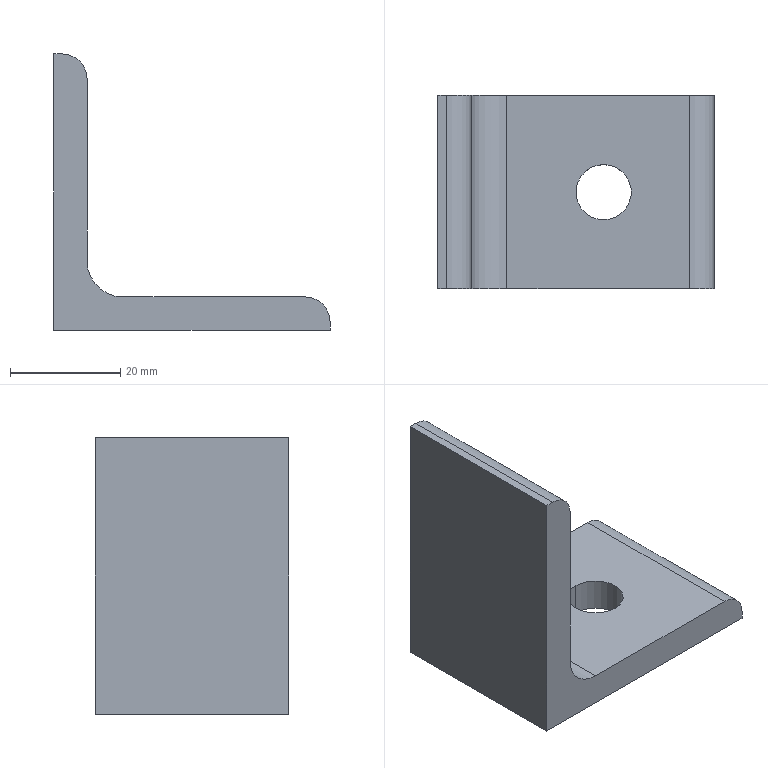Part | STEP file | [19]-2 | 1 solid | 13 faces | box 50 x 35 x 50 mm | volume 19282 mm3 | plane 8 | cylinder 5 | commonest cylinder face diameters 9 x2 10 x2 13 x1
STEP:
#1=CARTESIAN_POINT('',(30.,22.5,0.));
#2=VERTEX_POINT('',#1);
#3=CARTESIAN_POINT('',(30.,12.5,0.));
#4=VERTEX_POINT('',#3);
#5=CARTESIAN_POINT('',(30.,17.5,0.));
#6=DIRECTION('',(0.,0.,1.));
#7=DIRECTION('',(0.,-1.,0.));
#8=AXIS2_PLACEMENT_3D('',#5,#6,#7);
#9=CIRCLE('',#8,5.);
#10=EDGE_CURVE('',#2,#4,#9,.T.);
#11=ORIENTED_EDGE('',*,*,#10,.F.);
#12=CARTESIAN_POINT('',(30.,22.5,6.));
#13=VERTEX_POINT('',#12);
#14=CARTESIAN_POINT('',(30.,22.5,0.));
#15=DIRECTION('',(0.,0.,1.));
#16=VECTOR('',#15,1000.);
#17=LINE('',#14,#16);
#18=EDGE_CURVE('',#2,#13,#17,.T.);
#19=ORIENTED_EDGE('',*,*,#18,.T.);
#20=CARTESIAN_POINT('',(30.,12.5,6.));
#21=VERTEX_POINT('',#20);
#22=CARTESIAN_POINT('',(30.,17.5,6.));
#23=DIRECTION('',(0.,0.,-1.));
#24=DIRECTION('',(0.,1.,0.));
#25=AXIS2_PLACEMENT_3D('',#22,#23,#24);
#26=CIRCLE('',#25,5.);
#27=EDGE_CURVE('',#21,#13,#26,.T.);
#28=ORIENTED_EDGE('',*,*,#27,.F.);
#29=CARTESIAN_POINT('',(30.,12.5,0.));
#30=DIRECTION('',(0.,0.,1.));
#31=VECTOR('',#30,1000.);
#32=LINE('',#29,#31);
#33=EDGE_CURVE('',#4,#21,#32,.T.);
#34=ORIENTED_EDGE('',*,*,#33,.F.);
#35=EDGE_LOOP('',(#11,#19,#28,#34));
#36=FACE_OUTER_BOUND('',#35,.T.);
#37=CARTESIAN_POINT('',(30.,17.5,0.));
#38=DIRECTION('',(0.,0.,1.));
#39=DIRECTION('',(0.,-1.,0.));
#40=AXIS2_PLACEMENT_3D('',#37,#38,#39);
#41=CYLINDRICAL_SURFACE('',#40,5.);
#42=ADVANCED_FACE('',(#36),#41,.F.);
#43=CARTESIAN_POINT('',(30.,17.5,0.));
#44=DIRECTION('',(0.,0.,1.));
#45=DIRECTION('',(0.,-1.,0.));
#46=AXIS2_PLACEMENT_3D('',#43,#44,#45);
#47=CIRCLE('',#46,5.);
#48=EDGE_CURVE('',#4,#2,#47,.T.);
#49=ORIENTED_EDGE('',*,*,#48,.T.);
#50=ORIENTED_EDGE('',*,*,#10,.T.);
#51=EDGE_LOOP('',(#49,#50));
#52=FACE_BOUND('',#51,.T.);
#53=CARTESIAN_POINT('',(50.,0.,0.));
#54=VERTEX_POINT('',#53);
#55=CARTESIAN_POINT('',(0.,0.,0.));
#56=VERTEX_POINT('',#55);
#57=CARTESIAN_POINT('',(50.,0.,0.));
#58=DIRECTION('',(-1.,0.,0.));
#59=VECTOR('',#58,1000.);
#60=LINE('',#57,#59);
#61=EDGE_CURVE('',#54,#56,#60,.T.);
#62=ORIENTED_EDGE('',*,*,#61,.T.);
#63=CARTESIAN_POINT('',(0.,35.,0.));
#64=VERTEX_POINT('',#63);
#65=CARTESIAN_POINT('',(0.,35.,0.));
#66=DIRECTION('',(0.,-1.,0.));
#67=VECTOR('',#66,1000.);
#68=LINE('',#65,#67);
#69=EDGE_CURVE('',#64,#56,#68,.T.);
#70=ORIENTED_EDGE('',*,*,#69,.F.);
#71=CARTESIAN_POINT('',(50.,35.,0.));
#72=VERTEX_POINT('',#71);
#73=CARTESIAN_POINT('',(50.,35.,0.));
#74=DIRECTION('',(-1.,0.,0.));
#75=VECTOR('',#74,1000.);
#76=LINE('',#73,#75);
#77=EDGE_CURVE('',#72,#64,#76,.T.);
#78=ORIENTED_EDGE('',*,*,#77,.F.);
#79=CARTESIAN_POINT('',(50.,35.,0.));
#80=DIRECTION('',(0.,-1.,0.));
#81=VECTOR('',#80,1000.);
#82=LINE('',#79,#81);
#83=EDGE_CURVE('',#72,#54,#82,.T.);
#84=ORIENTED_EDGE('',*,*,#83,.T.);
#85=EDGE_LOOP('',(#62,#70,#78,#84));
#86=FACE_OUTER_BOUND('',#85,.T.);
#87=CARTESIAN_POINT('',(50.,35.,0.));
#88=DIRECTION('',(0.,0.,1.));
#89=DIRECTION('',(1.,0.,0.));
#90=AXIS2_PLACEMENT_3D('',#87,#88,#89);
#91=PLANE('',#90);
#92=ADVANCED_FACE('',(#52,#86),#91,.F.);
#93=CARTESIAN_POINT('',(0.,0.,50.));
#94=VERTEX_POINT('',#93);
#95=CARTESIAN_POINT('',(0.,0.,0.));
#96=DIRECTION('',(0.,0.,1.));
#97=VECTOR('',#96,1000.);
#98=LINE('',#95,#97);
#99=EDGE_CURVE('',#56,#94,#98,.T.);
#100=ORIENTED_EDGE('',*,*,#99,.T.);
#101=CARTESIAN_POINT('',(0.,35.,50.));
#102=VERTEX_POINT('',#101);
#103=CARTESIAN_POINT('',(0.,35.,50.));
#104=DIRECTION('',(0.,-1.,0.));
#105=VECTOR('',#104,1000.);
#106=LINE('',#103,#105);
#107=EDGE_CURVE('',#102,#94,#106,.T.);
#108=ORIENTED_EDGE('',*,*,#107,.F.);
#109=CARTESIAN_POINT('',(0.,35.,0.));
#110=DIRECTION('',(0.,0.,1.));
#111=VECTOR('',#110,1000.);
#112=LINE('',#109,#111);
#113=EDGE_CURVE('',#64,#102,#112,.T.);
#114=ORIENTED_EDGE('',*,*,#113,.F.);
#115=ORIENTED_EDGE('',*,*,#69,.T.);
#116=EDGE_LOOP('',(#100,#108,#114,#115));
#117=FACE_OUTER_BOUND('',#116,.T.);
#118=CARTESIAN_POINT('',(0.,35.,0.));
#119=DIRECTION('',(1.,0.,0.));
#120=DIRECTION('',(0.,0.,-1.));
#121=AXIS2_PLACEMENT_3D('',#118,#119,#120);
#122=PLANE('',#121);
#123=ADVANCED_FACE('',(#117),#122,.F.);
#124=CARTESIAN_POINT('',(1.5,0.,50.));
#125=VERTEX_POINT('',#124);
#126=CARTESIAN_POINT('',(0.,0.,50.));
#127=DIRECTION('',(1.,0.,0.));
#128=VECTOR('',#127,1000.);
#129=LINE('',#126,#128);
#130=EDGE_CURVE('',#94,#125,#129,.T.);
#131=ORIENTED_EDGE('',*,*,#130,.T.);
#132=CARTESIAN_POINT('',(1.5,35.,50.));
#133=VERTEX_POINT('',#132);
#134=CARTESIAN_POINT('',(1.5,35.,50.));
#135=DIRECTION('',(0.,-1.,0.));
#136=VECTOR('',#135,1000.);
#137=LINE('',#134,#136);
#138=EDGE_CURVE('',#133,#125,#137,.T.);
#139=ORIENTED_EDGE('',*,*,#138,.F.);
#140=CARTESIAN_POINT('',(0.,35.,50.));
#141=DIRECTION('',(1.,0.,0.));
#142=VECTOR('',#141,1000.);
#143=LINE('',#140,#142);
#144=EDGE_CURVE('',#102,#133,#143,.T.);
#145=ORIENTED_EDGE('',*,*,#144,.F.);
#146=ORIENTED_EDGE('',*,*,#107,.T.);
#147=EDGE_LOOP('',(#131,#139,#145,#146));
#148=FACE_OUTER_BOUND('',#147,.T.);
#149=CARTESIAN_POINT('',(0.,35.,50.));
#150=DIRECTION('',(0.,0.,-1.));
#151=DIRECTION('',(0.,1.,0.));
#152=AXIS2_PLACEMENT_3D('',#149,#150,#151);
#153=PLANE('',#152);
#154=ADVANCED_FACE('',(#148),#153,.F.);
#155=CARTESIAN_POINT('',(6.,0.,45.5));
#156=VERTEX_POINT('',#155);
#157=CARTESIAN_POINT('',(1.5,0.,45.5));
#158=DIRECTION('',(0.,1.,0.));
#159=DIRECTION('',(0.,0.,1.));
#160=AXIS2_PLACEMENT_3D('',#157,#158,#159);
#161=CIRCLE('',#160,4.5);
#162=EDGE_CURVE('',#125,#156,#161,.T.);
#163=ORIENTED_EDGE('',*,*,#162,.T.);
#164=CARTESIAN_POINT('',(6.,35.,45.5));
#165=VERTEX_POINT('',#164);
#166=CARTESIAN_POINT('',(6.,35.,45.5));
#167=DIRECTION('',(0.,-1.,0.));
#168=VECTOR('',#167,1000.);
#169=LINE('',#166,#168);
#170=EDGE_CURVE('',#165,#156,#169,.T.);
#171=ORIENTED_EDGE('',*,*,#170,.F.);
#172=CARTESIAN_POINT('',(1.5,35.,45.5));
#173=DIRECTION('',(0.,1.,0.));
#174=DIRECTION('',(0.,0.,1.));
#175=AXIS2_PLACEMENT_3D('',#172,#173,#174);
#176=CIRCLE('',#175,4.5);
#177=EDGE_CURVE('',#133,#165,#176,.T.);
#178=ORIENTED_EDGE('',*,*,#177,.F.);
#179=ORIENTED_EDGE('',*,*,#138,.T.);
#180=EDGE_LOOP('',(#163,#171,#178,#179));
#181=FACE_OUTER_BOUND('',#180,.T.);
#182=CARTESIAN_POINT('',(1.5,35.,45.5));
#183=DIRECTION('',(0.,-1.,0.));
#184=DIRECTION('',(0.,0.,-1.));
#185=AXIS2_PLACEMENT_3D('',#182,#183,#184);
#186=CYLINDRICAL_SURFACE('',#185,4.5);
#187=ADVANCED_FACE('',(#181),#186,.T.);
#188=CARTESIAN_POINT('',(6.,0.,12.5));
#189=VERTEX_POINT('',#188);
#190=CARTESIAN_POINT('',(6.,0.,45.5));
#191=DIRECTION('',(0.,0.,-1.));
#192=VECTOR('',#191,1000.);
#193=LINE('',#190,#192);
#194=EDGE_CURVE('',#156,#189,#193,.T.);
#195=ORIENTED_EDGE('',*,*,#194,.T.);
#196=CARTESIAN_POINT('',(6.,35.,12.5));
#197=VERTEX_POINT('',#196);
#198=CARTESIAN_POINT('',(6.,35.,12.5));
#199=DIRECTION('',(0.,-1.,0.));
#200=VECTOR('',#199,1000.);
#201=LINE('',#198,#200);
#202=EDGE_CURVE('',#197,#189,#201,.T.);
#203=ORIENTED_EDGE('',*,*,#202,.F.);
#204=CARTESIAN_POINT('',(6.,35.,45.5));
#205=DIRECTION('',(0.,0.,-1.));
#206=VECTOR('',#205,1000.);
#207=LINE('',#204,#206);
#208=EDGE_CURVE('',#165,#197,#207,.T.);
#209=ORIENTED_EDGE('',*,*,#208,.F.);
#210=ORIENTED_EDGE('',*,*,#170,.T.);
#211=EDGE_LOOP('',(#195,#203,#209,#210));
#212=FACE_OUTER_BOUND('',#211,.T.);
#213=CARTESIAN_POINT('',(6.,35.,45.5));
#214=DIRECTION('',(-1.,0.,0.));
#215=DIRECTION('',(0.,0.,1.));
#216=AXIS2_PLACEMENT_3D('',#213,#214,#215);
#217=PLANE('',#216);
#218=ADVANCED_FACE('',(#212),#217,.F.);
#219=CARTESIAN_POINT('',(12.5,0.,6.));
#220=VERTEX_POINT('',#219);
#221=CARTESIAN_POINT('',(12.5,0.,12.5));
#222=DIRECTION('',(0.,-1.,0.));
#223=DIRECTION('',(0.,0.,-1.));
#224=AXIS2_PLACEMENT_3D('',#221,#222,#223);
#225=CIRCLE('',#224,6.5);
#226=EDGE_CURVE('',#189,#220,#225,.T.);
#227=ORIENTED_EDGE('',*,*,#226,.T.);
#228=CARTESIAN_POINT('',(12.5,35.,6.));
#229=VERTEX_POINT('',#228);
#230=CARTESIAN_POINT('',(12.5,35.,6.));
#231=DIRECTION('',(0.,-1.,0.));
#232=VECTOR('',#231,1000.);
#233=LINE('',#230,#232);
#234=EDGE_CURVE('',#229,#220,#233,.T.);
#235=ORIENTED_EDGE('',*,*,#234,.F.);
#236=CARTESIAN_POINT('',(12.5,35.,12.5));
#237=DIRECTION('',(0.,-1.,0.));
#238=DIRECTION('',(0.,0.,-1.));
#239=AXIS2_PLACEMENT_3D('',#236,#237,#238);
#240=CIRCLE('',#239,6.5);
#241=EDGE_CURVE('',#197,#229,#240,.T.);
#242=ORIENTED_EDGE('',*,*,#241,.F.);
#243=ORIENTED_EDGE('',*,*,#202,.T.);
#244=EDGE_LOOP('',(#227,#235,#242,#243));
#245=FACE_OUTER_BOUND('',#244,.T.);
#246=CARTESIAN_POINT('',(12.5,35.,12.5));
#247=DIRECTION('',(0.,-1.,0.));
#248=DIRECTION('',(0.,0.,-1.));
#249=AXIS2_PLACEMENT_3D('',#246,#247,#248);
#250=CYLINDRICAL_SURFACE('',#249,6.5);
#251=ADVANCED_FACE('',(#245),#250,.F.);
#252=ORIENTED_EDGE('',*,*,#27,.T.);
#253=CARTESIAN_POINT('',(30.,17.5,6.));
#254=DIRECTION('',(0.,0.,-1.));
#255=DIRECTION('',(0.,1.,0.));
#256=AXIS2_PLACEMENT_3D('',#253,#254,#255);
#257=CIRCLE('',#256,5.);
#258=EDGE_CURVE('',#13,#21,#257,.T.);
#259=ORIENTED_EDGE('',*,*,#258,.T.);
#260=EDGE_LOOP('',(#252,#259));
#261=FACE_BOUND('',#260,.T.);
#262=CARTESIAN_POINT('',(45.5,0.,6.));
#263=VERTEX_POINT('',#262);
#264=CARTESIAN_POINT('',(12.5,0.,6.));
#265=DIRECTION('',(1.,0.,0.));
#266=VECTOR('',#265,1000.);
#267=LINE('',#264,#266);
#268=EDGE_CURVE('',#220,#263,#267,.T.);
#269=ORIENTED_EDGE('',*,*,#268,.T.);
#270=CARTESIAN_POINT('',(45.5,35.,6.));
#271=VERTEX_POINT('',#270);
#272=CARTESIAN_POINT('',(45.5,35.,6.));
#273=DIRECTION('',(0.,-1.,0.));
#274=VECTOR('',#273,1000.);
#275=LINE('',#272,#274);
#276=EDGE_CURVE('',#271,#263,#275,.T.);
#277=ORIENTED_EDGE('',*,*,#276,.F.);
#278=CARTESIAN_POINT('',(12.5,35.,6.));
#279=DIRECTION('',(1.,0.,0.));
#280=VECTOR('',#279,1000.);
#281=LINE('',#278,#280);
#282=EDGE_CURVE('',#229,#271,#281,.T.);
#283=ORIENTED_EDGE('',*,*,#282,.F.);
#284=ORIENTED_EDGE('',*,*,#234,.T.);
#285=EDGE_LOOP('',(#269,#277,#283,#284));
#286=FACE_OUTER_BOUND('',#285,.T.);
#287=CARTESIAN_POINT('',(12.5,35.,6.));
#288=DIRECTION('',(0.,0.,-1.));
#289=DIRECTION('',(-1.,0.,0.));
#290=AXIS2_PLACEMENT_3D('',#287,#288,#289);
#291=PLANE('',#290);
#292=ADVANCED_FACE('',(#261,#286),#291,.F.);
#293=CARTESIAN_POINT('',(50.,0.,1.5));
#294=VERTEX_POINT('',#293);
#295=CARTESIAN_POINT('',(45.5,0.,1.5));
#296=DIRECTION('',(0.,1.,0.));
#297=DIRECTION('',(0.,0.,1.));
#298=AXIS2_PLACEMENT_3D('',#295,#296,#297);
#299=CIRCLE('',#298,4.5);
#300=EDGE_CURVE('',#263,#294,#299,.T.);
#301=ORIENTED_EDGE('',*,*,#300,.T.);
#302=CARTESIAN_POINT('',(50.,35.,1.5));
#303=VERTEX_POINT('',#302);
#304=CARTESIAN_POINT('',(50.,35.,1.5));
#305=DIRECTION('',(0.,-1.,0.));
#306=VECTOR('',#305,1000.);
#307=LINE('',#304,#306);
#308=EDGE_CURVE('',#303,#294,#307,.T.);
#309=ORIENTED_EDGE('',*,*,#308,.F.);
#310=CARTESIAN_POINT('',(45.5,35.,1.5));
#311=DIRECTION('',(0.,1.,0.));
#312=DIRECTION('',(0.,0.,1.));
#313=AXIS2_PLACEMENT_3D('',#310,#311,#312);
#314=CIRCLE('',#313,4.5);
#315=EDGE_CURVE('',#271,#303,#314,.T.);
#316=ORIENTED_EDGE('',*,*,#315,.F.);
#317=ORIENTED_EDGE('',*,*,#276,.T.);
#318=EDGE_LOOP('',(#301,#309,#316,#317));
#319=FACE_OUTER_BOUND('',#318,.T.);
#320=CARTESIAN_POINT('',(45.5,35.,1.5));
#321=DIRECTION('',(0.,-1.,0.));
#322=DIRECTION('',(0.,0.,-1.));
#323=AXIS2_PLACEMENT_3D('',#320,#321,#322);
#324=CYLINDRICAL_SURFACE('',#323,4.5);
#325=ADVANCED_FACE('',(#319),#324,.T.);
#326=CARTESIAN_POINT('',(50.,0.,1.5));
#327=DIRECTION('',(0.,0.,-1.));
#328=VECTOR('',#327,1000.);
#329=LINE('',#326,#328);
#330=EDGE_CURVE('',#294,#54,#329,.T.);
#331=ORIENTED_EDGE('',*,*,#330,.T.);
#332=ORIENTED_EDGE('',*,*,#83,.F.);
#333=CARTESIAN_POINT('',(50.,35.,1.5));
#334=DIRECTION('',(0.,0.,-1.));
#335=VECTOR('',#334,1000.);
#336=LINE('',#333,#335);
#337=EDGE_CURVE('',#303,#72,#336,.T.);
#338=ORIENTED_EDGE('',*,*,#337,.F.);
#339=ORIENTED_EDGE('',*,*,#308,.T.);
#340=EDGE_LOOP('',(#331,#332,#338,#339));
#341=FACE_OUTER_BOUND('',#340,.T.);
#342=CARTESIAN_POINT('',(50.,35.,1.5));
#343=DIRECTION('',(-1.,0.,0.));
#344=DIRECTION('',(0.,-1.,0.));
#345=AXIS2_PLACEMENT_3D('',#342,#343,#344);
#346=PLANE('',#345);
#347=ADVANCED_FACE('',(#341),#346,.F.);
#348=ORIENTED_EDGE('',*,*,#77,.T.);
#349=ORIENTED_EDGE('',*,*,#113,.T.);
#350=ORIENTED_EDGE('',*,*,#144,.T.);
#351=ORIENTED_EDGE('',*,*,#177,.T.);
#352=ORIENTED_EDGE('',*,*,#208,.T.);
#353=ORIENTED_EDGE('',*,*,#241,.T.);
#354=ORIENTED_EDGE('',*,*,#282,.T.);
#355=ORIENTED_EDGE('',*,*,#315,.T.);
#356=ORIENTED_EDGE('',*,*,#337,.T.);
#357=EDGE_LOOP('',(#348,#349,#350,#351,#352,#353,#354,#355,#356));
#358=FACE_OUTER_BOUND('',#357,.T.);
#359=CARTESIAN_POINT('',(1.5,35.,45.5));
#360=DIRECTION('',(0.,1.,0.));
#361=DIRECTION('',(0.,0.,1.));
#362=AXIS2_PLACEMENT_3D('',#359,#360,#361);
#363=PLANE('',#362);
#364=ADVANCED_FACE('',(#358),#363,.T.);
#365=ORIENTED_EDGE('',*,*,#61,.F.);
#366=ORIENTED_EDGE('',*,*,#330,.F.);
#367=ORIENTED_EDGE('',*,*,#300,.F.);
#368=ORIENTED_EDGE('',*,*,#268,.F.);
#369=ORIENTED_EDGE('',*,*,#226,.F.);
#370=ORIENTED_EDGE('',*,*,#194,.F.);
#371=ORIENTED_EDGE('',*,*,#162,.F.);
#372=ORIENTED_EDGE('',*,*,#130,.F.);
#373=ORIENTED_EDGE('',*,*,#99,.F.);
#374=EDGE_LOOP('',(#365,#366,#367,#368,#369,#370,#371,#372,#373));
#375=FACE_OUTER_BOUND('',#374,.T.);
#376=CARTESIAN_POINT('',(1.5,0.,45.5));
#377=DIRECTION('',(0.,1.,0.));
#378=DIRECTION('',(0.,0.,1.));
#379=AXIS2_PLACEMENT_3D('',#376,#377,#378);
#380=PLANE('',#379);
#381=ADVANCED_FACE('',(#375),#380,.F.);
#382=ORIENTED_EDGE('',*,*,#18,.F.);
#383=ORIENTED_EDGE('',*,*,#48,.F.);
#384=ORIENTED_EDGE('',*,*,#33,.T.);
#385=ORIENTED_EDGE('',*,*,#258,.F.);
#386=EDGE_LOOP('',(#382,#383,#384,#385));
#387=FACE_OUTER_BOUND('',#386,.T.);
#388=CARTESIAN_POINT('',(30.,17.5,0.));
#389=DIRECTION('',(0.,0.,1.));
#390=DIRECTION('',(0.,-1.,0.));
#391=AXIS2_PLACEMENT_3D('',#388,#389,#390);
#392=CYLINDRICAL_SURFACE('',#391,5.);
#393=ADVANCED_FACE('',(#387),#392,.F.);
#394=CLOSED_SHELL('',(#42,#92,#123,#154,#187,#218,#251,#292,#325,#347,#364,#381,#393));
#395=MANIFOLD_SOLID_BREP('',#394);
#396=CARTESIAN_POINT('',(0.,0.,0.));
#397=DIRECTION('',(0.,0.,1.));
#398=DIRECTION('',(1.,0.,0.));
#399=AXIS2_PLACEMENT_3D('',#396,#397,#398);
#400=(LENGTH_UNIT()NAMED_UNIT(*)SI_UNIT(.MILLI.,.METRE.));
#401=UNCERTAINTY_MEASURE_WITH_UNIT(LENGTH_MEASURE(0.00001),#400,'','');
#402=(NAMED_UNIT(*)PLANE_ANGLE_UNIT()SI_UNIT($,.RADIAN.));
#403=(NAMED_UNIT(*)SI_UNIT($,.STERADIAN.)SOLID_ANGLE_UNIT());
#404=(GEOMETRIC_REPRESENTATION_CONTEXT(3)GLOBAL_UNCERTAINTY_ASSIGNED_CONTEXT((#401))GLOBAL_UNIT_ASSIGNED_CONTEXT((#400,#402,#403))REPRESENTATION_CONTEXT('',''));
#405=ADVANCED_BREP_SHAPE_REPRESENTATION('',(#395,#399),#404);